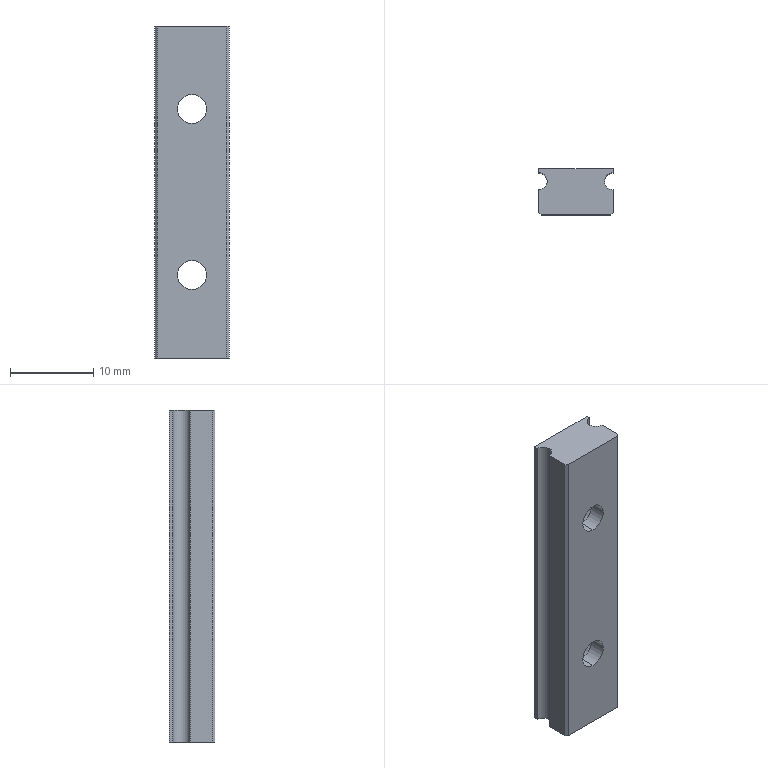Part | STEP file | 11-r_SEBL10_4011 | 1 solid | 23 faces | box 9 x 5.5 x 40 mm | volume 1604 mm3 | plane 12 | cylinder 11 | commonest cylinder face diameters 3.5 x4 6 x4 2.08 x3
STEP:
#1=CARTESIAN_POINT('',(0.,0.,28.25));
#2=VERTEX_POINT('',#1);
#3=CARTESIAN_POINT('',(0.,0.,31.75));
#4=VERTEX_POINT('',#3);
#5=CARTESIAN_POINT('',(0.,0.,30.));
#6=DIRECTION('',(0.,1.,0.));
#7=DIRECTION('',(0.,0.,1.));
#8=AXIS2_PLACEMENT_3D('',#5,#6,#7);
#9=CIRCLE('',#8,1.75);
#10=EDGE_CURVE('',#2,#4,#9,.T.);
#11=ORIENTED_EDGE('',*,*,#10,.F.);
#12=CARTESIAN_POINT('',(0.,2.,28.25));
#13=VERTEX_POINT('',#12);
#14=CARTESIAN_POINT('',(0.,0.,28.25));
#15=DIRECTION('',(0.,1.,0.));
#16=VECTOR('',#15,1000.);
#17=LINE('',#14,#16);
#18=EDGE_CURVE('',#2,#13,#17,.T.);
#19=ORIENTED_EDGE('',*,*,#18,.T.);
#20=CARTESIAN_POINT('',(0.,2.,31.75));
#21=VERTEX_POINT('',#20);
#22=CARTESIAN_POINT('',(0.,2.,30.));
#23=DIRECTION('',(0.,1.,0.));
#24=DIRECTION('',(0.,0.,1.));
#25=AXIS2_PLACEMENT_3D('',#22,#23,#24);
#26=CIRCLE('',#25,1.75);
#27=EDGE_CURVE('',#13,#21,#26,.T.);
#28=ORIENTED_EDGE('',*,*,#27,.T.);
#29=CARTESIAN_POINT('',(0.,0.,31.75));
#30=DIRECTION('',(0.,1.,0.));
#31=VECTOR('',#30,1000.);
#32=LINE('',#29,#31);
#33=EDGE_CURVE('',#4,#21,#32,.T.);
#34=ORIENTED_EDGE('',*,*,#33,.F.);
#35=EDGE_LOOP('',(#11,#19,#28,#34));
#36=FACE_OUTER_BOUND('',#35,.T.);
#37=CARTESIAN_POINT('',(0.,0.,30.));
#38=DIRECTION('',(0.,1.,0.));
#39=DIRECTION('',(0.,0.,1.));
#40=AXIS2_PLACEMENT_3D('',#37,#38,#39);
#41=CYLINDRICAL_SURFACE('',#40,1.75);
#42=ADVANCED_FACE('',(#36),#41,.F.);
#43=CARTESIAN_POINT('',(0.,2.,27.));
#44=VERTEX_POINT('',#43);
#45=CARTESIAN_POINT('',(0.,2.,33.));
#46=VERTEX_POINT('',#45);
#47=CARTESIAN_POINT('',(0.,2.,30.));
#48=DIRECTION('',(0.,1.,0.));
#49=DIRECTION('',(0.,0.,1.));
#50=AXIS2_PLACEMENT_3D('',#47,#48,#49);
#51=CIRCLE('',#50,3.);
#52=EDGE_CURVE('',#44,#46,#51,.T.);
#53=ORIENTED_EDGE('',*,*,#52,.F.);
#54=CARTESIAN_POINT('',(0.,5.5,27.));
#55=VERTEX_POINT('',#54);
#56=CARTESIAN_POINT('',(0.,0.,27.));
#57=DIRECTION('',(0.,1.,0.));
#58=VECTOR('',#57,1000.);
#59=LINE('',#56,#58);
#60=EDGE_CURVE('',#44,#55,#59,.T.);
#61=ORIENTED_EDGE('',*,*,#60,.T.);
#62=CARTESIAN_POINT('',(0.,5.5,33.));
#63=VERTEX_POINT('',#62);
#64=CARTESIAN_POINT('',(0.,5.5,30.));
#65=DIRECTION('',(0.,1.,0.));
#66=DIRECTION('',(0.,0.,1.));
#67=AXIS2_PLACEMENT_3D('',#64,#65,#66);
#68=CIRCLE('',#67,3.);
#69=EDGE_CURVE('',#55,#63,#68,.T.);
#70=ORIENTED_EDGE('',*,*,#69,.T.);
#71=CARTESIAN_POINT('',(0.,0.,33.));
#72=DIRECTION('',(0.,1.,0.));
#73=VECTOR('',#72,1000.);
#74=LINE('',#71,#73);
#75=EDGE_CURVE('',#46,#63,#74,.T.);
#76=ORIENTED_EDGE('',*,*,#75,.F.);
#77=EDGE_LOOP('',(#53,#61,#70,#76));
#78=FACE_OUTER_BOUND('',#77,.T.);
#79=CARTESIAN_POINT('',(0.,0.,30.));
#80=DIRECTION('',(0.,1.,0.));
#81=DIRECTION('',(0.,0.,1.));
#82=AXIS2_PLACEMENT_3D('',#79,#80,#81);
#83=CYLINDRICAL_SURFACE('',#82,3.);
#84=ADVANCED_FACE('',(#78),#83,.F.);
#85=CARTESIAN_POINT('',(0.,0.,8.25));
#86=VERTEX_POINT('',#85);
#87=CARTESIAN_POINT('',(0.,0.,11.75));
#88=VERTEX_POINT('',#87);
#89=CARTESIAN_POINT('',(0.,0.,10.));
#90=DIRECTION('',(0.,1.,0.));
#91=DIRECTION('',(0.,0.,1.));
#92=AXIS2_PLACEMENT_3D('',#89,#90,#91);
#93=CIRCLE('',#92,1.75);
#94=EDGE_CURVE('',#86,#88,#93,.T.);
#95=ORIENTED_EDGE('',*,*,#94,.F.);
#96=CARTESIAN_POINT('',(0.,2.,8.25));
#97=VERTEX_POINT('',#96);
#98=CARTESIAN_POINT('',(0.,0.,8.25));
#99=DIRECTION('',(0.,1.,0.));
#100=VECTOR('',#99,1000.);
#101=LINE('',#98,#100);
#102=EDGE_CURVE('',#86,#97,#101,.T.);
#103=ORIENTED_EDGE('',*,*,#102,.T.);
#104=CARTESIAN_POINT('',(0.,2.,11.75));
#105=VERTEX_POINT('',#104);
#106=CARTESIAN_POINT('',(0.,2.,10.));
#107=DIRECTION('',(0.,1.,0.));
#108=DIRECTION('',(0.,0.,1.));
#109=AXIS2_PLACEMENT_3D('',#106,#107,#108);
#110=CIRCLE('',#109,1.75);
#111=EDGE_CURVE('',#97,#105,#110,.T.);
#112=ORIENTED_EDGE('',*,*,#111,.T.);
#113=CARTESIAN_POINT('',(0.,0.,11.75));
#114=DIRECTION('',(0.,1.,0.));
#115=VECTOR('',#114,1000.);
#116=LINE('',#113,#115);
#117=EDGE_CURVE('',#88,#105,#116,.T.);
#118=ORIENTED_EDGE('',*,*,#117,.F.);
#119=EDGE_LOOP('',(#95,#103,#112,#118));
#120=FACE_OUTER_BOUND('',#119,.T.);
#121=CARTESIAN_POINT('',(0.,0.,10.));
#122=DIRECTION('',(0.,1.,0.));
#123=DIRECTION('',(0.,0.,1.));
#124=AXIS2_PLACEMENT_3D('',#121,#122,#123);
#125=CYLINDRICAL_SURFACE('',#124,1.75);
#126=ADVANCED_FACE('',(#120),#125,.F.);
#127=CARTESIAN_POINT('',(0.,2.,7.));
#128=VERTEX_POINT('',#127);
#129=CARTESIAN_POINT('',(0.,2.,13.));
#130=VERTEX_POINT('',#129);
#131=CARTESIAN_POINT('',(0.,2.,10.));
#132=DIRECTION('',(0.,1.,0.));
#133=DIRECTION('',(0.,0.,1.));
#134=AXIS2_PLACEMENT_3D('',#131,#132,#133);
#135=CIRCLE('',#134,3.);
#136=EDGE_CURVE('',#128,#130,#135,.T.);
#137=ORIENTED_EDGE('',*,*,#136,.F.);
#138=CARTESIAN_POINT('',(0.,5.5,7.));
#139=VERTEX_POINT('',#138);
#140=CARTESIAN_POINT('',(0.,0.,7.));
#141=DIRECTION('',(0.,1.,0.));
#142=VECTOR('',#141,1000.);
#143=LINE('',#140,#142);
#144=EDGE_CURVE('',#128,#139,#143,.T.);
#145=ORIENTED_EDGE('',*,*,#144,.T.);
#146=CARTESIAN_POINT('',(0.,5.5,13.));
#147=VERTEX_POINT('',#146);
#148=CARTESIAN_POINT('',(0.,5.5,10.));
#149=DIRECTION('',(0.,1.,0.));
#150=DIRECTION('',(0.,0.,1.));
#151=AXIS2_PLACEMENT_3D('',#148,#149,#150);
#152=CIRCLE('',#151,3.);
#153=EDGE_CURVE('',#139,#147,#152,.T.);
#154=ORIENTED_EDGE('',*,*,#153,.T.);
#155=CARTESIAN_POINT('',(0.,0.,13.));
#156=DIRECTION('',(0.,1.,0.));
#157=VECTOR('',#156,1000.);
#158=LINE('',#155,#157);
#159=EDGE_CURVE('',#130,#147,#158,.T.);
#160=ORIENTED_EDGE('',*,*,#159,.F.);
#161=EDGE_LOOP('',(#137,#145,#154,#160));
#162=FACE_OUTER_BOUND('',#161,.T.);
#163=CARTESIAN_POINT('',(0.,0.,10.));
#164=DIRECTION('',(0.,1.,0.));
#165=DIRECTION('',(0.,0.,1.));
#166=AXIS2_PLACEMENT_3D('',#163,#164,#165);
#167=CYLINDRICAL_SURFACE('',#166,3.);
#168=ADVANCED_FACE('',(#162),#167,.F.);
#169=CARTESIAN_POINT('',(3.46,4.,40.));
#170=VERTEX_POINT('',#169);
#171=CARTESIAN_POINT('',(4.5,5.04,40.));
#172=VERTEX_POINT('',#171);
#173=CARTESIAN_POINT('',(4.5,4.,40.));
#174=DIRECTION('',(0.,0.,-1.));
#175=DIRECTION('',(-1.,0.,0.));
#176=AXIS2_PLACEMENT_3D('',#173,#174,#175);
#177=CIRCLE('',#176,1.04);
#178=EDGE_CURVE('',#170,#172,#177,.T.);
#179=ORIENTED_EDGE('',*,*,#178,.F.);
#180=CARTESIAN_POINT('',(3.46,4.,0.));
#181=VERTEX_POINT('',#180);
#182=CARTESIAN_POINT('',(3.46,4.,40.));
#183=DIRECTION('',(0.,0.,-1.));
#184=VECTOR('',#183,1000.);
#185=LINE('',#182,#184);
#186=EDGE_CURVE('',#170,#181,#185,.T.);
#187=ORIENTED_EDGE('',*,*,#186,.T.);
#188=CARTESIAN_POINT('',(4.5,5.04,0.));
#189=VERTEX_POINT('',#188);
#190=CARTESIAN_POINT('',(4.5,4.,0.));
#191=DIRECTION('',(0.,0.,-1.));
#192=DIRECTION('',(-1.,0.,0.));
#193=AXIS2_PLACEMENT_3D('',#190,#191,#192);
#194=CIRCLE('',#193,1.04);
#195=EDGE_CURVE('',#181,#189,#194,.T.);
#196=ORIENTED_EDGE('',*,*,#195,.T.);
#197=CARTESIAN_POINT('',(4.5,5.04,40.));
#198=DIRECTION('',(0.,0.,-1.));
#199=VECTOR('',#198,1000.);
#200=LINE('',#197,#199);
#201=EDGE_CURVE('',#172,#189,#200,.T.);
#202=ORIENTED_EDGE('',*,*,#201,.F.);
#203=EDGE_LOOP('',(#179,#187,#196,#202));
#204=FACE_OUTER_BOUND('',#203,.T.);
#205=CARTESIAN_POINT('',(4.5,4.,40.));
#206=DIRECTION('',(0.,0.,-1.));
#207=DIRECTION('',(-1.,0.,0.));
#208=AXIS2_PLACEMENT_3D('',#205,#206,#207);
#209=CYLINDRICAL_SURFACE('',#208,1.04);
#210=ADVANCED_FACE('',(#204),#209,.F.);
#211=CARTESIAN_POINT('',(0.,5.5,30.));
#212=DIRECTION('',(0.,1.,0.));
#213=DIRECTION('',(0.,0.,1.));
#214=AXIS2_PLACEMENT_3D('',#211,#212,#213);
#215=CIRCLE('',#214,3.);
#216=EDGE_CURVE('',#63,#55,#215,.T.);
#217=ORIENTED_EDGE('',*,*,#216,.F.);
#218=ORIENTED_EDGE('',*,*,#69,.F.);
#219=EDGE_LOOP('',(#217,#218));
#220=FACE_BOUND('',#219,.T.);
#221=CARTESIAN_POINT('',(0.,5.5,10.));
#222=DIRECTION('',(0.,1.,0.));
#223=DIRECTION('',(0.,0.,1.));
#224=AXIS2_PLACEMENT_3D('',#221,#222,#223);
#225=CIRCLE('',#224,3.);
#226=EDGE_CURVE('',#147,#139,#225,.T.);
#227=ORIENTED_EDGE('',*,*,#226,.F.);
#228=ORIENTED_EDGE('',*,*,#153,.F.);
#229=EDGE_LOOP('',(#227,#228));
#230=FACE_BOUND('',#229,.T.);
#231=CARTESIAN_POINT('',(4.5,5.5,0.));
#232=VERTEX_POINT('',#231);
#233=CARTESIAN_POINT('',(-4.5,5.5,0.));
#234=VERTEX_POINT('',#233);
#235=CARTESIAN_POINT('',(4.5,5.5,0.));
#236=DIRECTION('',(-1.,0.,0.));
#237=VECTOR('',#236,1000.);
#238=LINE('',#235,#237);
#239=EDGE_CURVE('',#232,#234,#238,.T.);
#240=ORIENTED_EDGE('',*,*,#239,.T.);
#241=CARTESIAN_POINT('',(-4.5,5.5,40.));
#242=VERTEX_POINT('',#241);
#243=CARTESIAN_POINT('',(-4.5,5.5,40.));
#244=DIRECTION('',(0.,0.,-1.));
#245=VECTOR('',#244,1000.);
#246=LINE('',#243,#245);
#247=EDGE_CURVE('',#242,#234,#246,.T.);
#248=ORIENTED_EDGE('',*,*,#247,.F.);
#249=CARTESIAN_POINT('',(4.5,5.5,40.));
#250=VERTEX_POINT('',#249);
#251=CARTESIAN_POINT('',(4.5,5.5,40.));
#252=DIRECTION('',(-1.,0.,0.));
#253=VECTOR('',#252,1000.);
#254=LINE('',#251,#253);
#255=EDGE_CURVE('',#250,#242,#254,.T.);
#256=ORIENTED_EDGE('',*,*,#255,.F.);
#257=CARTESIAN_POINT('',(4.5,5.5,40.));
#258=DIRECTION('',(0.,0.,-1.));
#259=VECTOR('',#258,1000.);
#260=LINE('',#257,#259);
#261=EDGE_CURVE('',#250,#232,#260,.T.);
#262=ORIENTED_EDGE('',*,*,#261,.T.);
#263=EDGE_LOOP('',(#240,#248,#256,#262));
#264=FACE_OUTER_BOUND('',#263,.T.);
#265=CARTESIAN_POINT('',(4.5,5.5,40.));
#266=DIRECTION('',(0.,-1.,0.));
#267=DIRECTION('',(0.,0.,-1.));
#268=AXIS2_PLACEMENT_3D('',#265,#266,#267);
#269=PLANE('',#268);
#270=ADVANCED_FACE('',(#220,#230,#264),#269,.F.);
#271=CARTESIAN_POINT('',(-4.5,5.04,0.));
#272=VERTEX_POINT('',#271);
#273=CARTESIAN_POINT('',(-4.5,5.5,0.));
#274=DIRECTION('',(0.,-1.,0.));
#275=VECTOR('',#274,1000.);
#276=LINE('',#273,#275);
#277=EDGE_CURVE('',#234,#272,#276,.T.);
#278=ORIENTED_EDGE('',*,*,#277,.T.);
#279=CARTESIAN_POINT('',(-4.5,5.04,40.));
#280=VERTEX_POINT('',#279);
#281=CARTESIAN_POINT('',(-4.5,5.04,40.));
#282=DIRECTION('',(0.,0.,-1.));
#283=VECTOR('',#282,1000.);
#284=LINE('',#281,#283);
#285=EDGE_CURVE('',#280,#272,#284,.T.);
#286=ORIENTED_EDGE('',*,*,#285,.F.);
#287=CARTESIAN_POINT('',(-4.5,5.5,40.));
#288=DIRECTION('',(0.,-1.,0.));
#289=VECTOR('',#288,1000.);
#290=LINE('',#287,#289);
#291=EDGE_CURVE('',#242,#280,#290,.T.);
#292=ORIENTED_EDGE('',*,*,#291,.F.);
#293=ORIENTED_EDGE('',*,*,#247,.T.);
#294=EDGE_LOOP('',(#278,#286,#292,#293));
#295=FACE_OUTER_BOUND('',#294,.T.);
#296=CARTESIAN_POINT('',(-4.5,5.5,40.));
#297=DIRECTION('',(1.,0.,0.));
#298=DIRECTION('',(0.,0.,-1.));
#299=AXIS2_PLACEMENT_3D('',#296,#297,#298);
#300=PLANE('',#299);
#301=ADVANCED_FACE('',(#295),#300,.F.);
#302=CARTESIAN_POINT('',(-4.5,2.96,0.));
#303=VERTEX_POINT('',#302);
#304=CARTESIAN_POINT('',(-4.5,4.,0.));
#305=DIRECTION('',(0.,0.,-1.));
#306=DIRECTION('',(-1.,0.,0.));
#307=AXIS2_PLACEMENT_3D('',#304,#305,#306);
#308=CIRCLE('',#307,1.04);
#309=EDGE_CURVE('',#272,#303,#308,.T.);
#310=ORIENTED_EDGE('',*,*,#309,.T.);
#311=CARTESIAN_POINT('',(-4.5,2.96,40.));
#312=VERTEX_POINT('',#311);
#313=CARTESIAN_POINT('',(-4.5,2.96,40.));
#314=DIRECTION('',(0.,0.,-1.));
#315=VECTOR('',#314,1000.);
#316=LINE('',#313,#315);
#317=EDGE_CURVE('',#312,#303,#316,.T.);
#318=ORIENTED_EDGE('',*,*,#317,.F.);
#319=CARTESIAN_POINT('',(-4.5,4.,40.));
#320=DIRECTION('',(0.,0.,-1.));
#321=DIRECTION('',(-1.,0.,0.));
#322=AXIS2_PLACEMENT_3D('',#319,#320,#321);
#323=CIRCLE('',#322,1.04);
#324=EDGE_CURVE('',#280,#312,#323,.T.);
#325=ORIENTED_EDGE('',*,*,#324,.F.);
#326=ORIENTED_EDGE('',*,*,#285,.T.);
#327=EDGE_LOOP('',(#310,#318,#325,#326));
#328=FACE_OUTER_BOUND('',#327,.T.);
#329=CARTESIAN_POINT('',(-4.5,4.,40.));
#330=DIRECTION('',(0.,0.,-1.));
#331=DIRECTION('',(-1.,0.,0.));
#332=AXIS2_PLACEMENT_3D('',#329,#330,#331);
#333=CYLINDRICAL_SURFACE('',#332,1.04);
#334=ADVANCED_FACE('',(#328),#333,.F.);
#335=CARTESIAN_POINT('',(-4.5,0.3,0.));
#336=VERTEX_POINT('',#335);
#337=CARTESIAN_POINT('',(-4.5,2.96,0.));
#338=DIRECTION('',(0.,-1.,0.));
#339=VECTOR('',#338,1000.);
#340=LINE('',#337,#339);
#341=EDGE_CURVE('',#303,#336,#340,.T.);
#342=ORIENTED_EDGE('',*,*,#341,.T.);
#343=CARTESIAN_POINT('',(-4.5,0.3,40.));
#344=VERTEX_POINT('',#343);
#345=CARTESIAN_POINT('',(-4.5,0.3,40.));
#346=DIRECTION('',(0.,0.,-1.));
#347=VECTOR('',#346,1000.);
#348=LINE('',#345,#347);
#349=EDGE_CURVE('',#344,#336,#348,.T.);
#350=ORIENTED_EDGE('',*,*,#349,.F.);
#351=CARTESIAN_POINT('',(-4.5,2.96,40.));
#352=DIRECTION('',(0.,-1.,0.));
#353=VECTOR('',#352,1000.);
#354=LINE('',#351,#353);
#355=EDGE_CURVE('',#312,#344,#354,.T.);
#356=ORIENTED_EDGE('',*,*,#355,.F.);
#357=ORIENTED_EDGE('',*,*,#317,.T.);
#358=EDGE_LOOP('',(#342,#350,#356,#357));
#359=FACE_OUTER_BOUND('',#358,.T.);
#360=CARTESIAN_POINT('',(-4.5,2.96,40.));
#361=DIRECTION('',(1.,0.,0.));
#362=DIRECTION('',(0.,0.,-1.));
#363=AXIS2_PLACEMENT_3D('',#360,#361,#362);
#364=PLANE('',#363);
#365=ADVANCED_FACE('',(#359),#364,.F.);
#366=CARTESIAN_POINT('',(-4.2,0.,0.));
#367=VERTEX_POINT('',#366);
#368=CARTESIAN_POINT('',(-4.5,0.3,0.));
#369=DIRECTION('',(0.7071,-0.7071,0.));
#370=VECTOR('',#369,1000.);
#371=LINE('',#368,#370);
#372=EDGE_CURVE('',#336,#367,#371,.T.);
#373=ORIENTED_EDGE('',*,*,#372,.T.);
#374=CARTESIAN_POINT('',(-4.2,0.,40.));
#375=VERTEX_POINT('',#374);
#376=CARTESIAN_POINT('',(-4.2,0.,40.));
#377=DIRECTION('',(0.,0.,-1.));
#378=VECTOR('',#377,1000.);
#379=LINE('',#376,#378);
#380=EDGE_CURVE('',#375,#367,#379,.T.);
#381=ORIENTED_EDGE('',*,*,#380,.F.);
#382=CARTESIAN_POINT('',(-4.5,0.3,40.));
#383=DIRECTION('',(0.7071,-0.7071,0.));
#384=VECTOR('',#383,1000.);
#385=LINE('',#382,#384);
#386=EDGE_CURVE('',#344,#375,#385,.T.);
#387=ORIENTED_EDGE('',*,*,#386,.F.);
#388=ORIENTED_EDGE('',*,*,#349,.T.);
#389=EDGE_LOOP('',(#373,#381,#387,#388));
#390=FACE_OUTER_BOUND('',#389,.T.);
#391=CARTESIAN_POINT('',(-4.5,0.3,40.));
#392=DIRECTION('',(0.7071,0.7071,0.));
#393=DIRECTION('',(-0.7071,0.7071,0.));
#394=AXIS2_PLACEMENT_3D('',#391,#392,#393);
#395=PLANE('',#394);
#396=ADVANCED_FACE('',(#390),#395,.F.);
#397=CARTESIAN_POINT('',(0.,0.,30.));
#398=DIRECTION('',(0.,1.,0.));
#399=DIRECTION('',(0.,0.,1.));
#400=AXIS2_PLACEMENT_3D('',#397,#398,#399);
#401=CIRCLE('',#400,1.75);
#402=EDGE_CURVE('',#4,#2,#401,.T.);
#403=ORIENTED_EDGE('',*,*,#402,.T.);
#404=ORIENTED_EDGE('',*,*,#10,.T.);
#405=EDGE_LOOP('',(#403,#404));
#406=FACE_BOUND('',#405,.T.);
#407=CARTESIAN_POINT('',(0.,0.,10.));
#408=DIRECTION('',(0.,1.,0.));
#409=DIRECTION('',(0.,0.,1.));
#410=AXIS2_PLACEMENT_3D('',#407,#408,#409);
#411=CIRCLE('',#410,1.75);
#412=EDGE_CURVE('',#88,#86,#411,.T.);
#413=ORIENTED_EDGE('',*,*,#412,.T.);
#414=ORIENTED_EDGE('',*,*,#94,.T.);
#415=EDGE_LOOP('',(#413,#414));
#416=FACE_BOUND('',#415,.T.);
#417=CARTESIAN_POINT('',(4.2,0.,0.));
#418=VERTEX_POINT('',#417);
#419=CARTESIAN_POINT('',(-4.2,0.,0.));
#420=DIRECTION('',(1.,0.,0.));
#421=VECTOR('',#420,1000.);
#422=LINE('',#419,#421);
#423=EDGE_CURVE('',#367,#418,#422,.T.);
#424=ORIENTED_EDGE('',*,*,#423,.T.);
#425=CARTESIAN_POINT('',(4.2,0.,40.));
#426=VERTEX_POINT('',#425);
#427=CARTESIAN_POINT('',(4.2,0.,40.));
#428=DIRECTION('',(0.,0.,-1.));
#429=VECTOR('',#428,1000.);
#430=LINE('',#427,#429);
#431=EDGE_CURVE('',#426,#418,#430,.T.);
#432=ORIENTED_EDGE('',*,*,#431,.F.);
#433=CARTESIAN_POINT('',(-4.2,0.,40.));
#434=DIRECTION('',(1.,0.,0.));
#435=VECTOR('',#434,1000.);
#436=LINE('',#433,#435);
#437=EDGE_CURVE('',#375,#426,#436,.T.);
#438=ORIENTED_EDGE('',*,*,#437,.F.);
#439=ORIENTED_EDGE('',*,*,#380,.T.);
#440=EDGE_LOOP('',(#424,#432,#438,#439));
#441=FACE_OUTER_BOUND('',#440,.T.);
#442=CARTESIAN_POINT('',(-4.2,0.,40.));
#443=DIRECTION('',(0.,1.,0.));
#444=DIRECTION('',(0.,0.,1.));
#445=AXIS2_PLACEMENT_3D('',#442,#443,#444);
#446=PLANE('',#445);
#447=ADVANCED_FACE('',(#406,#416,#441),#446,.F.);
#448=CARTESIAN_POINT('',(4.5,0.3,0.));
#449=VERTEX_POINT('',#448);
#450=CARTESIAN_POINT('',(4.2,0.,0.));
#451=DIRECTION('',(0.7071,0.7071,0.));
#452=VECTOR('',#451,1000.);
#453=LINE('',#450,#452);
#454=EDGE_CURVE('',#418,#449,#453,.T.);
#455=ORIENTED_EDGE('',*,*,#454,.T.);
#456=CARTESIAN_POINT('',(4.5,0.3,40.));
#457=VERTEX_POINT('',#456);
#458=CARTESIAN_POINT('',(4.5,0.3,40.));
#459=DIRECTION('',(0.,0.,-1.));
#460=VECTOR('',#459,1000.);
#461=LINE('',#458,#460);
#462=EDGE_CURVE('',#457,#449,#461,.T.);
#463=ORIENTED_EDGE('',*,*,#462,.F.);
#464=CARTESIAN_POINT('',(4.2,0.,40.));
#465=DIRECTION('',(0.7071,0.7071,0.));
#466=VECTOR('',#465,1000.);
#467=LINE('',#464,#466);
#468=EDGE_CURVE('',#426,#457,#467,.T.);
#469=ORIENTED_EDGE('',*,*,#468,.F.);
#470=ORIENTED_EDGE('',*,*,#431,.T.);
#471=EDGE_LOOP('',(#455,#463,#469,#470));
#472=FACE_OUTER_BOUND('',#471,.T.);
#473=CARTESIAN_POINT('',(4.2,0.,40.));
#474=DIRECTION('',(-0.7071,0.7071,0.));
#475=DIRECTION('',(-0.7071,-0.7071,0.));
#476=AXIS2_PLACEMENT_3D('',#473,#474,#475);
#477=PLANE('',#476);
#478=ADVANCED_FACE('',(#472),#477,.F.);
#479=CARTESIAN_POINT('',(4.5,2.96,0.));
#480=VERTEX_POINT('',#479);
#481=CARTESIAN_POINT('',(4.5,0.3,0.));
#482=DIRECTION('',(0.,1.,0.));
#483=VECTOR('',#482,1000.);
#484=LINE('',#481,#483);
#485=EDGE_CURVE('',#449,#480,#484,.T.);
#486=ORIENTED_EDGE('',*,*,#485,.T.);
#487=CARTESIAN_POINT('',(4.5,2.96,40.));
#488=VERTEX_POINT('',#487);
#489=CARTESIAN_POINT('',(4.5,2.96,40.));
#490=DIRECTION('',(0.,0.,-1.));
#491=VECTOR('',#490,1000.);
#492=LINE('',#489,#491);
#493=EDGE_CURVE('',#488,#480,#492,.T.);
#494=ORIENTED_EDGE('',*,*,#493,.F.);
#495=CARTESIAN_POINT('',(4.5,0.3,40.));
#496=DIRECTION('',(0.,1.,0.));
#497=VECTOR('',#496,1000.);
#498=LINE('',#495,#497);
#499=EDGE_CURVE('',#457,#488,#498,.T.);
#500=ORIENTED_EDGE('',*,*,#499,.F.);
#501=ORIENTED_EDGE('',*,*,#462,.T.);
#502=EDGE_LOOP('',(#486,#494,#500,#501));
#503=FACE_OUTER_BOUND('',#502,.T.);
#504=CARTESIAN_POINT('',(4.5,0.3,40.));
#505=DIRECTION('',(-1.,0.,0.));
#506=DIRECTION('',(0.,0.,1.));
#507=AXIS2_PLACEMENT_3D('',#504,#505,#506);
#508=PLANE('',#507);
#509=ADVANCED_FACE('',(#503),#508,.F.);
#510=ORIENTED_EDGE('',*,*,#186,.F.);
#511=CARTESIAN_POINT('',(4.5,4.,40.));
#512=DIRECTION('',(0.,0.,-1.));
#513=DIRECTION('',(-1.,0.,0.));
#514=AXIS2_PLACEMENT_3D('',#511,#512,#513);
#515=CIRCLE('',#514,1.04);
#516=EDGE_CURVE('',#488,#170,#515,.T.);
#517=ORIENTED_EDGE('',*,*,#516,.F.);
#518=ORIENTED_EDGE('',*,*,#493,.T.);
#519=CARTESIAN_POINT('',(4.5,4.,0.));
#520=DIRECTION('',(0.,0.,-1.));
#521=DIRECTION('',(-1.,0.,0.));
#522=AXIS2_PLACEMENT_3D('',#519,#520,#521);
#523=CIRCLE('',#522,1.04);
#524=EDGE_CURVE('',#480,#181,#523,.T.);
#525=ORIENTED_EDGE('',*,*,#524,.T.);
#526=EDGE_LOOP('',(#510,#517,#518,#525));
#527=FACE_OUTER_BOUND('',#526,.T.);
#528=CARTESIAN_POINT('',(4.5,4.,40.));
#529=DIRECTION('',(0.,0.,-1.));
#530=DIRECTION('',(-1.,0.,0.));
#531=AXIS2_PLACEMENT_3D('',#528,#529,#530);
#532=CYLINDRICAL_SURFACE('',#531,1.04);
#533=ADVANCED_FACE('',(#527),#532,.F.);
#534=CARTESIAN_POINT('',(4.5,5.04,0.));
#535=DIRECTION('',(0.,1.,0.));
#536=VECTOR('',#535,1000.);
#537=LINE('',#534,#536);
#538=EDGE_CURVE('',#189,#232,#537,.T.);
#539=ORIENTED_EDGE('',*,*,#538,.T.);
#540=ORIENTED_EDGE('',*,*,#261,.F.);
#541=CARTESIAN_POINT('',(4.5,5.04,40.));
#542=DIRECTION('',(0.,1.,0.));
#543=VECTOR('',#542,1000.);
#544=LINE('',#541,#543);
#545=EDGE_CURVE('',#172,#250,#544,.T.);
#546=ORIENTED_EDGE('',*,*,#545,.F.);
#547=ORIENTED_EDGE('',*,*,#201,.T.);
#548=EDGE_LOOP('',(#539,#540,#546,#547));
#549=FACE_OUTER_BOUND('',#548,.T.);
#550=CARTESIAN_POINT('',(4.5,5.04,40.));
#551=DIRECTION('',(-1.,0.,0.));
#552=DIRECTION('',(0.,0.,1.));
#553=AXIS2_PLACEMENT_3D('',#550,#551,#552);
#554=PLANE('',#553);
#555=ADVANCED_FACE('',(#549),#554,.F.);
#556=ORIENTED_EDGE('',*,*,#255,.T.);
#557=ORIENTED_EDGE('',*,*,#291,.T.);
#558=ORIENTED_EDGE('',*,*,#324,.T.);
#559=ORIENTED_EDGE('',*,*,#355,.T.);
#560=ORIENTED_EDGE('',*,*,#386,.T.);
#561=ORIENTED_EDGE('',*,*,#437,.T.);
#562=ORIENTED_EDGE('',*,*,#468,.T.);
#563=ORIENTED_EDGE('',*,*,#499,.T.);
#564=ORIENTED_EDGE('',*,*,#516,.T.);
#565=ORIENTED_EDGE('',*,*,#178,.T.);
#566=ORIENTED_EDGE('',*,*,#545,.T.);
#567=EDGE_LOOP('',(#556,#557,#558,#559,#560,#561,#562,#563,#564,#565,#566));
#568=FACE_OUTER_BOUND('',#567,.T.);
#569=CARTESIAN_POINT('',(-4.5,4.,40.));
#570=DIRECTION('',(0.,0.,-1.));
#571=DIRECTION('',(-1.,0.,0.));
#572=AXIS2_PLACEMENT_3D('',#569,#570,#571);
#573=PLANE('',#572);
#574=ADVANCED_FACE('',(#568),#573,.F.);
#575=ORIENTED_EDGE('',*,*,#239,.F.);
#576=ORIENTED_EDGE('',*,*,#538,.F.);
#577=ORIENTED_EDGE('',*,*,#195,.F.);
#578=ORIENTED_EDGE('',*,*,#524,.F.);
#579=ORIENTED_EDGE('',*,*,#485,.F.);
#580=ORIENTED_EDGE('',*,*,#454,.F.);
#581=ORIENTED_EDGE('',*,*,#423,.F.);
#582=ORIENTED_EDGE('',*,*,#372,.F.);
#583=ORIENTED_EDGE('',*,*,#341,.F.);
#584=ORIENTED_EDGE('',*,*,#309,.F.);
#585=ORIENTED_EDGE('',*,*,#277,.F.);
#586=EDGE_LOOP('',(#575,#576,#577,#578,#579,#580,#581,#582,#583,#584,#585));
#587=FACE_OUTER_BOUND('',#586,.T.);
#588=CARTESIAN_POINT('',(-4.5,4.,0.));
#589=DIRECTION('',(0.,0.,-1.));
#590=DIRECTION('',(-1.,0.,0.));
#591=AXIS2_PLACEMENT_3D('',#588,#589,#590);
#592=PLANE('',#591);
#593=ADVANCED_FACE('',(#587),#592,.T.);
#594=ORIENTED_EDGE('',*,*,#144,.F.);
#595=CARTESIAN_POINT('',(0.,2.,10.));
#596=DIRECTION('',(0.,1.,0.));
#597=DIRECTION('',(0.,0.,1.));
#598=AXIS2_PLACEMENT_3D('',#595,#596,#597);
#599=CIRCLE('',#598,3.);
#600=EDGE_CURVE('',#130,#128,#599,.T.);
#601=ORIENTED_EDGE('',*,*,#600,.F.);
#602=ORIENTED_EDGE('',*,*,#159,.T.);
#603=ORIENTED_EDGE('',*,*,#226,.T.);
#604=EDGE_LOOP('',(#594,#601,#602,#603));
#605=FACE_OUTER_BOUND('',#604,.T.);
#606=CARTESIAN_POINT('',(0.,0.,10.));
#607=DIRECTION('',(0.,1.,0.));
#608=DIRECTION('',(0.,0.,1.));
#609=AXIS2_PLACEMENT_3D('',#606,#607,#608);
#610=CYLINDRICAL_SURFACE('',#609,3.);
#611=ADVANCED_FACE('',(#605),#610,.F.);
#612=ORIENTED_EDGE('',*,*,#600,.T.);
#613=ORIENTED_EDGE('',*,*,#136,.T.);
#614=EDGE_LOOP('',(#612,#613));
#615=FACE_OUTER_BOUND('',#614,.T.);
#616=CARTESIAN_POINT('',(0.,2.,10.));
#617=DIRECTION('',(0.,1.,0.));
#618=DIRECTION('',(0.,0.,1.));
#619=AXIS2_PLACEMENT_3D('',#616,#617,#618);
#620=CIRCLE('',#619,1.75);
#621=EDGE_CURVE('',#105,#97,#620,.T.);
#622=ORIENTED_EDGE('',*,*,#621,.F.);
#623=ORIENTED_EDGE('',*,*,#111,.F.);
#624=EDGE_LOOP('',(#622,#623));
#625=FACE_BOUND('',#624,.T.);
#626=CARTESIAN_POINT('',(0.,2.,7.));
#627=DIRECTION('',(0.,1.,0.));
#628=DIRECTION('',(0.,0.,1.));
#629=AXIS2_PLACEMENT_3D('',#626,#627,#628);
#630=PLANE('',#629);
#631=ADVANCED_FACE('',(#615,#625),#630,.T.);
#632=ORIENTED_EDGE('',*,*,#102,.F.);
#633=ORIENTED_EDGE('',*,*,#412,.F.);
#634=ORIENTED_EDGE('',*,*,#117,.T.);
#635=ORIENTED_EDGE('',*,*,#621,.T.);
#636=EDGE_LOOP('',(#632,#633,#634,#635));
#637=FACE_OUTER_BOUND('',#636,.T.);
#638=CARTESIAN_POINT('',(0.,0.,10.));
#639=DIRECTION('',(0.,1.,0.));
#640=DIRECTION('',(0.,0.,1.));
#641=AXIS2_PLACEMENT_3D('',#638,#639,#640);
#642=CYLINDRICAL_SURFACE('',#641,1.75);
#643=ADVANCED_FACE('',(#637),#642,.F.);
#644=ORIENTED_EDGE('',*,*,#60,.F.);
#645=CARTESIAN_POINT('',(0.,2.,30.));
#646=DIRECTION('',(0.,1.,0.));
#647=DIRECTION('',(0.,0.,1.));
#648=AXIS2_PLACEMENT_3D('',#645,#646,#647);
#649=CIRCLE('',#648,3.);
#650=EDGE_CURVE('',#46,#44,#649,.T.);
#651=ORIENTED_EDGE('',*,*,#650,.F.);
#652=ORIENTED_EDGE('',*,*,#75,.T.);
#653=ORIENTED_EDGE('',*,*,#216,.T.);
#654=EDGE_LOOP('',(#644,#651,#652,#653));
#655=FACE_OUTER_BOUND('',#654,.T.);
#656=CARTESIAN_POINT('',(0.,0.,30.));
#657=DIRECTION('',(0.,1.,0.));
#658=DIRECTION('',(0.,0.,1.));
#659=AXIS2_PLACEMENT_3D('',#656,#657,#658);
#660=CYLINDRICAL_SURFACE('',#659,3.);
#661=ADVANCED_FACE('',(#655),#660,.F.);
#662=ORIENTED_EDGE('',*,*,#650,.T.);
#663=ORIENTED_EDGE('',*,*,#52,.T.);
#664=EDGE_LOOP('',(#662,#663));
#665=FACE_OUTER_BOUND('',#664,.T.);
#666=CARTESIAN_POINT('',(0.,2.,30.));
#667=DIRECTION('',(0.,1.,0.));
#668=DIRECTION('',(0.,0.,1.));
#669=AXIS2_PLACEMENT_3D('',#666,#667,#668);
#670=CIRCLE('',#669,1.75);
#671=EDGE_CURVE('',#21,#13,#670,.T.);
#672=ORIENTED_EDGE('',*,*,#671,.F.);
#673=ORIENTED_EDGE('',*,*,#27,.F.);
#674=EDGE_LOOP('',(#672,#673));
#675=FACE_BOUND('',#674,.T.);
#676=CARTESIAN_POINT('',(0.,2.,27.));
#677=DIRECTION('',(0.,1.,0.));
#678=DIRECTION('',(0.,0.,1.));
#679=AXIS2_PLACEMENT_3D('',#676,#677,#678);
#680=PLANE('',#679);
#681=ADVANCED_FACE('',(#665,#675),#680,.T.);
#682=ORIENTED_EDGE('',*,*,#18,.F.);
#683=ORIENTED_EDGE('',*,*,#402,.F.);
#684=ORIENTED_EDGE('',*,*,#33,.T.);
#685=ORIENTED_EDGE('',*,*,#671,.T.);
#686=EDGE_LOOP('',(#682,#683,#684,#685));
#687=FACE_OUTER_BOUND('',#686,.T.);
#688=CARTESIAN_POINT('',(0.,0.,30.));
#689=DIRECTION('',(0.,1.,0.));
#690=DIRECTION('',(0.,0.,1.));
#691=AXIS2_PLACEMENT_3D('',#688,#689,#690);
#692=CYLINDRICAL_SURFACE('',#691,1.75);
#693=ADVANCED_FACE('',(#687),#692,.F.);
#694=CLOSED_SHELL('',(#42,#84,#126,#168,#210,#270,#301,#334,#365,#396,#447,#478,#509,#533,#555,#574,#593,#611,#631,#643,#661,#681,#693));
#695=MANIFOLD_SOLID_BREP('',#694);
#696=CARTESIAN_POINT('',(0.,0.,0.));
#697=DIRECTION('',(0.,0.,1.));
#698=DIRECTION('',(1.,0.,0.));
#699=AXIS2_PLACEMENT_3D('',#696,#697,#698);
#700=(LENGTH_UNIT()NAMED_UNIT(*)SI_UNIT(.MILLI.,.METRE.));
#701=UNCERTAINTY_MEASURE_WITH_UNIT(LENGTH_MEASURE(0.00001),#700,'','');
#702=(NAMED_UNIT(*)PLANE_ANGLE_UNIT()SI_UNIT($,.RADIAN.));
#703=(NAMED_UNIT(*)SI_UNIT($,.STERADIAN.)SOLID_ANGLE_UNIT());
#704=(GEOMETRIC_REPRESENTATION_CONTEXT(3)GLOBAL_UNCERTAINTY_ASSIGNED_CONTEXT((#701))GLOBAL_UNIT_ASSIGNED_CONTEXT((#700,#702,#703))REPRESENTATION_CONTEXT('',''));
#705=ADVANCED_BREP_SHAPE_REPRESENTATION('',(#695,#699),#704);